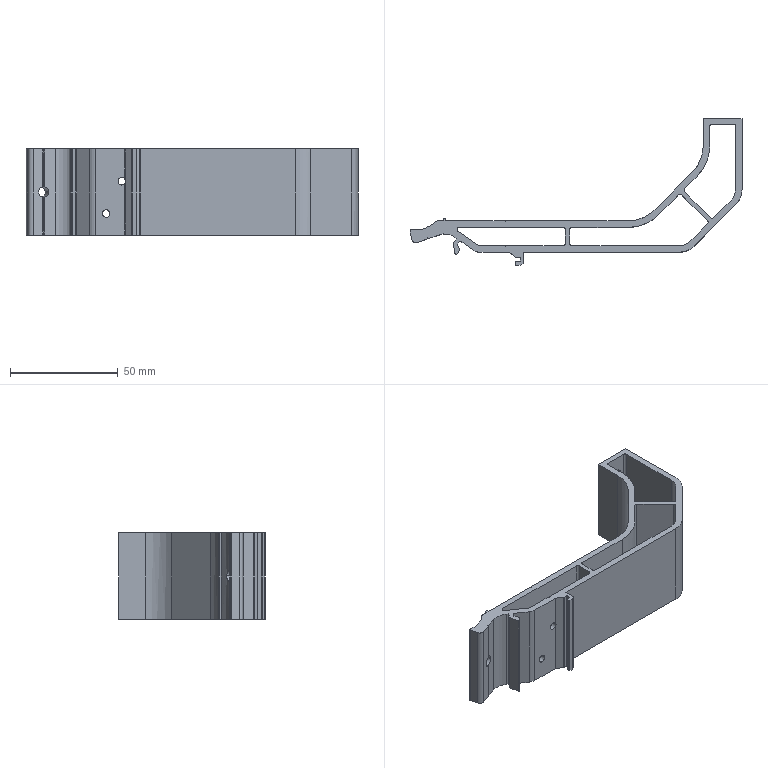Part | STEP file | 51E-01214JG10 | 1 solid | 130 faces | box 154.2 x 68 x 40 mm | volume 48290 mm3 | cylinder 67 | plane 63 | commonest cylinder face diameters 0.6 x21 2 x15 10 x5 3.5 x4 6.5 x4 0.4 x2